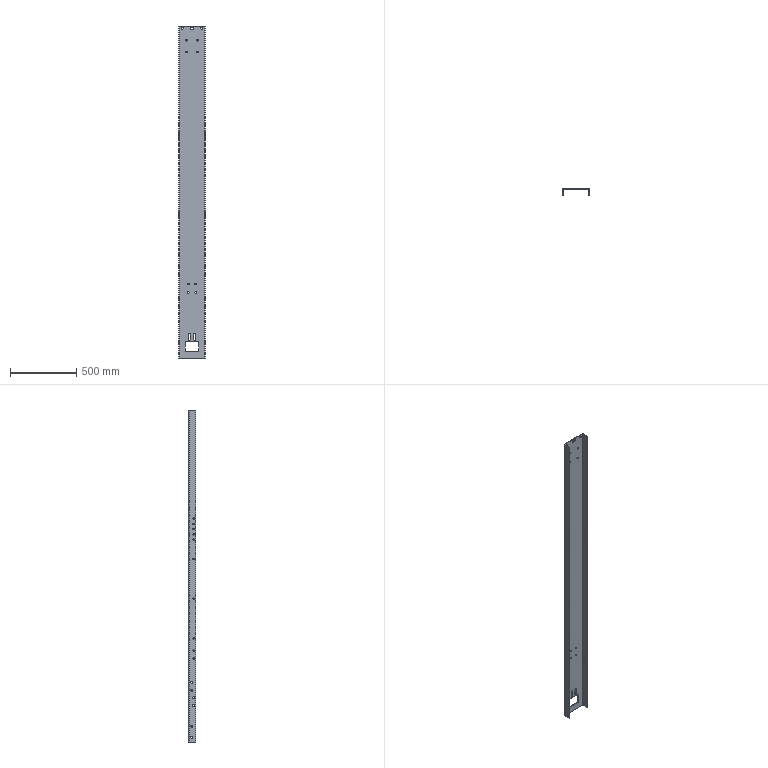Part | 1 solid | 123 faces | box 200 x 55 x 2510 mm | volume 2948034 mm3 | cylinder 95 | plane 28 | commonest cylinder face diameters 11 x40 14 x32 12.5 x8 13 x8 20 x3 2 x2